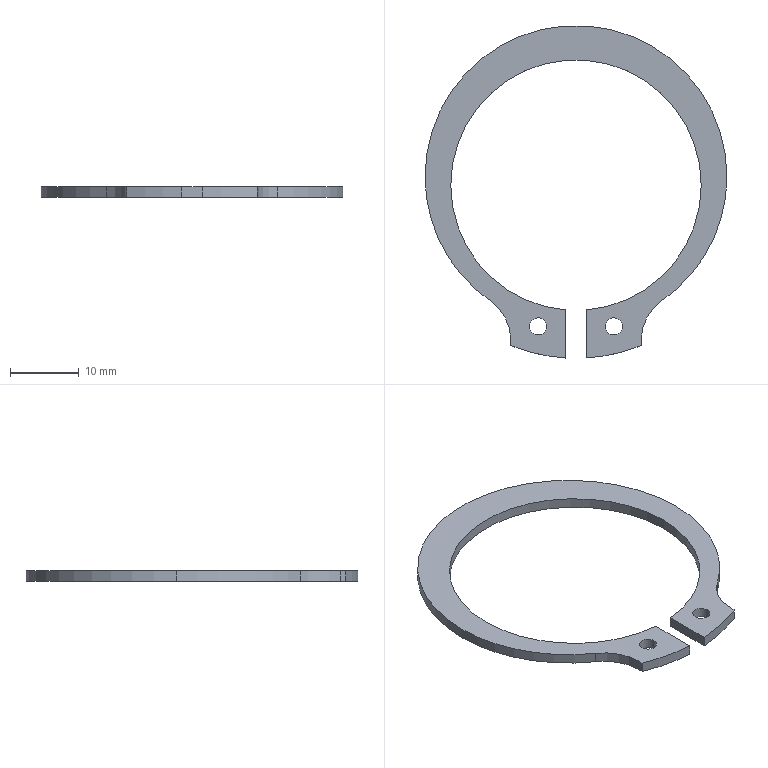Part | SolidWorks | features BaseBody 1 | 1 solid | 20 faces | box 44 x 48.435 x 1.5 mm | volume 802.613 mm3 | cylinder 14 | plane 6 | commonest cylinder face diameters 2.5 x4 36.5 x3 44 x3 14 x2 50.46 x2
STEP:
#1=CARTESIAN_POINT('',(22.,0.,-1.5));
#2=VERTEX_POINT('',#1);
#3=CARTESIAN_POINT('',(-22.,0.,-1.5));
#4=VERTEX_POINT('',#3);
#5=CARTESIAN_POINT('',(0.,0.,-1.5));
#6=DIRECTION('',(0.,0.,1.));
#7=DIRECTION('',(1.,0.,0.));
#8=AXIS2_PLACEMENT_3D('',#5,#6,#7);
#9=CIRCLE('',#8,22.);
#10=EDGE_CURVE('',#2,#4,#9,.T.);
#11=ORIENTED_EDGE('',*,*,#10,.T.);
#12=CARTESIAN_POINT('',(-22.,0.,0.));
#13=VERTEX_POINT('',#12);
#14=CARTESIAN_POINT('',(-22.,0.,-1.5));
#15=DIRECTION('',(0.,0.,1.));
#16=VECTOR('',#15,1000.);
#17=LINE('',#14,#16);
#18=EDGE_CURVE('',#4,#13,#17,.T.);
#19=ORIENTED_EDGE('',*,*,#18,.T.);
#20=CARTESIAN_POINT('',(22.,0.,0.));
#21=VERTEX_POINT('',#20);
#22=CARTESIAN_POINT('',(0.,0.,0.));
#23=DIRECTION('',(0.,0.,-1.));
#24=DIRECTION('',(1.,0.,0.));
#25=AXIS2_PLACEMENT_3D('',#22,#23,#24);
#26=CIRCLE('',#25,22.);
#27=EDGE_CURVE('',#13,#21,#26,.T.);
#28=ORIENTED_EDGE('',*,*,#27,.T.);
#29=CARTESIAN_POINT('',(22.,0.,-1.5));
#30=DIRECTION('',(0.,0.,1.));
#31=VECTOR('',#30,1000.);
#32=LINE('',#29,#31);
#33=EDGE_CURVE('',#2,#21,#32,.T.);
#34=ORIENTED_EDGE('',*,*,#33,.F.);
#35=EDGE_LOOP('',(#11,#19,#28,#34));
#36=FACE_OUTER_BOUND('',#35,.T.);
#37=CARTESIAN_POINT('',(0.,0.,-1.5));
#38=DIRECTION('',(0.,0.,1.));
#39=DIRECTION('',(1.,0.,0.));
#40=AXIS2_PLACEMENT_3D('',#37,#38,#39);
#41=CYLINDRICAL_SURFACE('',#40,22.);
#42=ADVANCED_FACE('',(#36),#41,.T.);
#43=CARTESIAN_POINT('',(12.517,-18.092,-1.5));
#44=VERTEX_POINT('',#43);
#45=CARTESIAN_POINT('',(0.,0.,-1.5));
#46=DIRECTION('',(0.,0.,1.));
#47=DIRECTION('',(1.,0.,0.));
#48=AXIS2_PLACEMENT_3D('',#45,#46,#47);
#49=CIRCLE('',#48,22.);
#50=EDGE_CURVE('',#44,#2,#49,.T.);
#51=ORIENTED_EDGE('',*,*,#50,.T.);
#52=ORIENTED_EDGE('',*,*,#33,.T.);
#53=CARTESIAN_POINT('',(12.517,-18.092,0.));
#54=VERTEX_POINT('',#53);
#55=CARTESIAN_POINT('',(0.,0.,0.));
#56=DIRECTION('',(0.,0.,-1.));
#57=DIRECTION('',(1.,0.,0.));
#58=AXIS2_PLACEMENT_3D('',#55,#56,#57);
#59=CIRCLE('',#58,22.);
#60=EDGE_CURVE('',#21,#54,#59,.T.);
#61=ORIENTED_EDGE('',*,*,#60,.T.);
#62=CARTESIAN_POINT('',(12.517,-18.092,-1.5));
#63=DIRECTION('',(0.,0.,-1.));
#64=VECTOR('',#63,1000.);
#65=LINE('',#62,#64);
#66=EDGE_CURVE('',#54,#44,#65,.T.);
#67=ORIENTED_EDGE('',*,*,#66,.T.);
#68=EDGE_LOOP('',(#51,#52,#61,#67));
#69=FACE_OUTER_BOUND('',#68,.T.);
#70=CARTESIAN_POINT('',(0.,0.,-1.5));
#71=DIRECTION('',(0.,0.,1.));
#72=DIRECTION('',(1.,0.,0.));
#73=AXIS2_PLACEMENT_3D('',#70,#71,#72);
#74=CYLINDRICAL_SURFACE('',#73,22.);
#75=ADVANCED_FACE('',(#69),#74,.T.);
#76=CARTESIAN_POINT('',(-1.5,-19.438,-1.5));
#77=VERTEX_POINT('',#76);
#78=CARTESIAN_POINT('',(-18.25,-1.25,-1.5));
#79=VERTEX_POINT('',#78);
#80=CARTESIAN_POINT('',(0.,-1.25,-1.5));
#81=DIRECTION('',(0.,0.,-1.));
#82=DIRECTION('',(1.,0.,0.));
#83=AXIS2_PLACEMENT_3D('',#80,#81,#82);
#84=CIRCLE('',#83,18.25);
#85=EDGE_CURVE('',#77,#79,#84,.T.);
#86=ORIENTED_EDGE('',*,*,#85,.T.);
#87=CARTESIAN_POINT('',(-18.25,-1.25,0.));
#88=VERTEX_POINT('',#87);
#89=CARTESIAN_POINT('',(-18.25,-1.25,-1.5));
#90=DIRECTION('',(0.,0.,1.));
#91=VECTOR('',#90,1000.);
#92=LINE('',#89,#91);
#93=EDGE_CURVE('',#79,#88,#92,.T.);
#94=ORIENTED_EDGE('',*,*,#93,.T.);
#95=CARTESIAN_POINT('',(-1.5,-19.438,0.));
#96=VERTEX_POINT('',#95);
#97=CARTESIAN_POINT('',(0.,-1.25,0.));
#98=DIRECTION('',(0.,0.,-1.));
#99=DIRECTION('',(1.,0.,0.));
#100=AXIS2_PLACEMENT_3D('',#97,#98,#99);
#101=CIRCLE('',#100,18.25);
#102=EDGE_CURVE('',#96,#88,#101,.T.);
#103=ORIENTED_EDGE('',*,*,#102,.F.);
#104=CARTESIAN_POINT('',(-1.5,-19.438,-1.5));
#105=DIRECTION('',(0.,0.,1.));
#106=VECTOR('',#105,1000.);
#107=LINE('',#104,#106);
#108=EDGE_CURVE('',#77,#96,#107,.T.);
#109=ORIENTED_EDGE('',*,*,#108,.F.);
#110=EDGE_LOOP('',(#86,#94,#103,#109));
#111=FACE_OUTER_BOUND('',#110,.T.);
#112=CARTESIAN_POINT('',(0.,-1.25,-1.5));
#113=DIRECTION('',(0.,0.,1.));
#114=DIRECTION('',(1.,0.,0.));
#115=AXIS2_PLACEMENT_3D('',#112,#113,#114);
#116=CYLINDRICAL_SURFACE('',#115,18.25);
#117=ADVANCED_FACE('',(#111),#116,.F.);
#118=ORIENTED_EDGE('',*,*,#93,.F.);
#119=CARTESIAN_POINT('',(18.25,-1.25,-1.5));
#120=VERTEX_POINT('',#119);
#121=CARTESIAN_POINT('',(0.,-1.25,-1.5));
#122=DIRECTION('',(0.,0.,-1.));
#123=DIRECTION('',(1.,0.,0.));
#124=AXIS2_PLACEMENT_3D('',#121,#122,#123);
#125=CIRCLE('',#124,18.25);
#126=EDGE_CURVE('',#79,#120,#125,.T.);
#127=ORIENTED_EDGE('',*,*,#126,.T.);
#128=CARTESIAN_POINT('',(18.25,-1.25,0.));
#129=VERTEX_POINT('',#128);
#130=CARTESIAN_POINT('',(18.25,-1.25,-1.5));
#131=DIRECTION('',(0.,0.,1.));
#132=VECTOR('',#131,1000.);
#133=LINE('',#130,#132);
#134=EDGE_CURVE('',#120,#129,#133,.T.);
#135=ORIENTED_EDGE('',*,*,#134,.T.);
#136=CARTESIAN_POINT('',(0.,-1.25,0.));
#137=DIRECTION('',(0.,0.,-1.));
#138=DIRECTION('',(1.,0.,0.));
#139=AXIS2_PLACEMENT_3D('',#136,#137,#138);
#140=CIRCLE('',#139,18.25);
#141=EDGE_CURVE('',#88,#129,#140,.T.);
#142=ORIENTED_EDGE('',*,*,#141,.F.);
#143=EDGE_LOOP('',(#118,#127,#135,#142));
#144=FACE_OUTER_BOUND('',#143,.T.);
#145=CARTESIAN_POINT('',(0.,-1.25,-1.5));
#146=DIRECTION('',(0.,0.,1.));
#147=DIRECTION('',(1.,0.,0.));
#148=AXIS2_PLACEMENT_3D('',#145,#146,#147);
#149=CYLINDRICAL_SURFACE('',#148,18.25);
#150=ADVANCED_FACE('',(#144),#149,.F.);
#151=CARTESIAN_POINT('',(-4.25,-21.828,-1.5));
#152=VERTEX_POINT('',#151);
#153=CARTESIAN_POINT('',(-6.75,-21.828,-1.5));
#154=VERTEX_POINT('',#153);
#155=CARTESIAN_POINT('',(-5.5,-21.828,-1.5));
#156=DIRECTION('',(0.,0.,-1.));
#157=DIRECTION('',(1.,0.,0.));
#158=AXIS2_PLACEMENT_3D('',#155,#156,#157);
#159=CIRCLE('',#158,1.25);
#160=EDGE_CURVE('',#152,#154,#159,.T.);
#161=ORIENTED_EDGE('',*,*,#160,.T.);
#162=CARTESIAN_POINT('',(-6.75,-21.828,0.));
#163=VERTEX_POINT('',#162);
#164=CARTESIAN_POINT('',(-6.75,-21.828,-1.5));
#165=DIRECTION('',(0.,0.,1.));
#166=VECTOR('',#165,1000.);
#167=LINE('',#164,#166);
#168=EDGE_CURVE('',#154,#163,#167,.T.);
#169=ORIENTED_EDGE('',*,*,#168,.T.);
#170=CARTESIAN_POINT('',(-4.25,-21.828,0.));
#171=VERTEX_POINT('',#170);
#172=CARTESIAN_POINT('',(-5.5,-21.828,0.));
#173=DIRECTION('',(0.,0.,-1.));
#174=DIRECTION('',(1.,0.,0.));
#175=AXIS2_PLACEMENT_3D('',#172,#173,#174);
#176=CIRCLE('',#175,1.25);
#177=EDGE_CURVE('',#171,#163,#176,.T.);
#178=ORIENTED_EDGE('',*,*,#177,.F.);
#179=CARTESIAN_POINT('',(-4.25,-21.828,-1.5));
#180=DIRECTION('',(0.,0.,1.));
#181=VECTOR('',#180,1000.);
#182=LINE('',#179,#181);
#183=EDGE_CURVE('',#152,#171,#182,.T.);
#184=ORIENTED_EDGE('',*,*,#183,.F.);
#185=EDGE_LOOP('',(#161,#169,#178,#184));
#186=FACE_OUTER_BOUND('',#185,.T.);
#187=CARTESIAN_POINT('',(-5.5,-21.828,-1.5));
#188=DIRECTION('',(0.,0.,1.));
#189=DIRECTION('',(1.,0.,0.));
#190=AXIS2_PLACEMENT_3D('',#187,#188,#189);
#191=CYLINDRICAL_SURFACE('',#190,1.25);
#192=ADVANCED_FACE('',(#186),#191,.F.);
#193=CARTESIAN_POINT('',(6.75,-21.828,-1.5));
#194=VERTEX_POINT('',#193);
#195=CARTESIAN_POINT('',(4.25,-21.828,-1.5));
#196=VERTEX_POINT('',#195);
#197=CARTESIAN_POINT('',(5.5,-21.828,-1.5));
#198=DIRECTION('',(0.,0.,-1.));
#199=DIRECTION('',(1.,0.,0.));
#200=AXIS2_PLACEMENT_3D('',#197,#198,#199);
#201=CIRCLE('',#200,1.25);
#202=EDGE_CURVE('',#194,#196,#201,.T.);
#203=ORIENTED_EDGE('',*,*,#202,.T.);
#204=CARTESIAN_POINT('',(4.25,-21.828,0.));
#205=VERTEX_POINT('',#204);
#206=CARTESIAN_POINT('',(4.25,-21.828,-1.5));
#207=DIRECTION('',(0.,0.,1.));
#208=VECTOR('',#207,1000.);
#209=LINE('',#206,#208);
#210=EDGE_CURVE('',#196,#205,#209,.T.);
#211=ORIENTED_EDGE('',*,*,#210,.T.);
#212=CARTESIAN_POINT('',(6.75,-21.828,0.));
#213=VERTEX_POINT('',#212);
#214=CARTESIAN_POINT('',(5.5,-21.828,0.));
#215=DIRECTION('',(0.,0.,-1.));
#216=DIRECTION('',(1.,0.,0.));
#217=AXIS2_PLACEMENT_3D('',#214,#215,#216);
#218=CIRCLE('',#217,1.25);
#219=EDGE_CURVE('',#213,#205,#218,.T.);
#220=ORIENTED_EDGE('',*,*,#219,.F.);
#221=CARTESIAN_POINT('',(6.75,-21.828,-1.5));
#222=DIRECTION('',(0.,0.,1.));
#223=VECTOR('',#222,1000.);
#224=LINE('',#221,#223);
#225=EDGE_CURVE('',#194,#213,#224,.T.);
#226=ORIENTED_EDGE('',*,*,#225,.F.);
#227=EDGE_LOOP('',(#203,#211,#220,#226));
#228=FACE_OUTER_BOUND('',#227,.T.);
#229=CARTESIAN_POINT('',(5.5,-21.828,-1.5));
#230=DIRECTION('',(0.,0.,1.));
#231=DIRECTION('',(1.,0.,0.));
#232=AXIS2_PLACEMENT_3D('',#229,#230,#231);
#233=CYLINDRICAL_SURFACE('',#232,1.25);
#234=ADVANCED_FACE('',(#228),#233,.F.);
#235=CARTESIAN_POINT('',(9.5,-23.848,-1.5));
#236=VERTEX_POINT('',#235);
#237=CARTESIAN_POINT('',(16.5,-23.848,-1.5));
#238=DIRECTION('',(0.,0.,-1.));
#239=DIRECTION('',(1.,0.,0.));
#240=AXIS2_PLACEMENT_3D('',#237,#238,#239);
#241=CIRCLE('',#240,7.);
#242=EDGE_CURVE('',#236,#44,#241,.T.);
#243=ORIENTED_EDGE('',*,*,#242,.F.);
#244=CARTESIAN_POINT('',(9.5,-24.623,-1.5));
#245=VERTEX_POINT('',#244);
#246=CARTESIAN_POINT('',(9.5,0.,-1.5));
#247=DIRECTION('',(0.,1.,0.));
#248=VECTOR('',#247,1000.);
#249=LINE('',#246,#248);
#250=EDGE_CURVE('',#245,#236,#249,.T.);
#251=ORIENTED_EDGE('',*,*,#250,.F.);
#252=CARTESIAN_POINT('',(1.5,-26.435,-1.5));
#253=VERTEX_POINT('',#252);
#254=CARTESIAN_POINT('',(0.,-1.25,-1.5));
#255=DIRECTION('',(0.,0.,1.));
#256=DIRECTION('',(1.,0.,0.));
#257=AXIS2_PLACEMENT_3D('',#254,#255,#256);
#258=CIRCLE('',#257,25.23);
#259=EDGE_CURVE('',#253,#245,#258,.T.);
#260=ORIENTED_EDGE('',*,*,#259,.F.);
#261=CARTESIAN_POINT('',(1.5,-19.438,-1.5));
#262=VERTEX_POINT('',#261);
#263=CARTESIAN_POINT('',(1.5,0.,-1.5));
#264=DIRECTION('',(0.,-1.,0.));
#265=VECTOR('',#264,1000.);
#266=LINE('',#263,#265);
#267=EDGE_CURVE('',#262,#253,#266,.T.);
#268=ORIENTED_EDGE('',*,*,#267,.F.);
#269=CARTESIAN_POINT('',(0.,-1.25,-1.5));
#270=DIRECTION('',(0.,0.,-1.));
#271=DIRECTION('',(1.,0.,0.));
#272=AXIS2_PLACEMENT_3D('',#269,#270,#271);
#273=CIRCLE('',#272,18.25);
#274=EDGE_CURVE('',#120,#262,#273,.T.);
#275=ORIENTED_EDGE('',*,*,#274,.F.);
#276=ORIENTED_EDGE('',*,*,#126,.F.);
#277=ORIENTED_EDGE('',*,*,#85,.F.);
#278=CARTESIAN_POINT('',(-1.5,-26.435,-1.5));
#279=VERTEX_POINT('',#278);
#280=CARTESIAN_POINT('',(-1.5,0.,-1.5));
#281=DIRECTION('',(0.,1.,0.));
#282=VECTOR('',#281,1000.);
#283=LINE('',#280,#282);
#284=EDGE_CURVE('',#279,#77,#283,.T.);
#285=ORIENTED_EDGE('',*,*,#284,.F.);
#286=CARTESIAN_POINT('',(-9.5,-24.623,-1.5));
#287=VERTEX_POINT('',#286);
#288=CARTESIAN_POINT('',(0.,-1.25,-1.5));
#289=DIRECTION('',(0.,0.,1.));
#290=DIRECTION('',(1.,0.,0.));
#291=AXIS2_PLACEMENT_3D('',#288,#289,#290);
#292=CIRCLE('',#291,25.23);
#293=EDGE_CURVE('',#287,#279,#292,.T.);
#294=ORIENTED_EDGE('',*,*,#293,.F.);
#295=CARTESIAN_POINT('',(-9.5,-23.848,-1.5));
#296=VERTEX_POINT('',#295);
#297=CARTESIAN_POINT('',(-9.5,0.,-1.5));
#298=DIRECTION('',(0.,-1.,0.));
#299=VECTOR('',#298,1000.);
#300=LINE('',#297,#299);
#301=EDGE_CURVE('',#296,#287,#300,.T.);
#302=ORIENTED_EDGE('',*,*,#301,.F.);
#303=CARTESIAN_POINT('',(-12.517,-18.092,-1.5));
#304=VERTEX_POINT('',#303);
#305=CARTESIAN_POINT('',(-16.5,-23.848,-1.5));
#306=DIRECTION('',(0.,0.,-1.));
#307=DIRECTION('',(1.,0.,0.));
#308=AXIS2_PLACEMENT_3D('',#305,#306,#307);
#309=CIRCLE('',#308,7.);
#310=EDGE_CURVE('',#304,#296,#309,.T.);
#311=ORIENTED_EDGE('',*,*,#310,.F.);
#312=CARTESIAN_POINT('',(0.,0.,-1.5));
#313=DIRECTION('',(0.,0.,1.));
#314=DIRECTION('',(1.,0.,0.));
#315=AXIS2_PLACEMENT_3D('',#312,#313,#314);
#316=CIRCLE('',#315,22.);
#317=EDGE_CURVE('',#4,#304,#316,.T.);
#318=ORIENTED_EDGE('',*,*,#317,.F.);
#319=ORIENTED_EDGE('',*,*,#10,.F.);
#320=ORIENTED_EDGE('',*,*,#50,.F.);
#321=EDGE_LOOP('',(#243,#251,#260,#268,#275,#276,#277,#285,#294,#302,#311,#318,#319,#320));
#322=FACE_OUTER_BOUND('',#321,.T.);
#323=ORIENTED_EDGE('',*,*,#160,.F.);
#324=CARTESIAN_POINT('',(-5.5,-21.828,-1.5));
#325=DIRECTION('',(0.,0.,-1.));
#326=DIRECTION('',(1.,0.,0.));
#327=AXIS2_PLACEMENT_3D('',#324,#325,#326);
#328=CIRCLE('',#327,1.25);
#329=EDGE_CURVE('',#154,#152,#328,.T.);
#330=ORIENTED_EDGE('',*,*,#329,.F.);
#331=EDGE_LOOP('',(#323,#330));
#332=FACE_BOUND('',#331,.T.);
#333=ORIENTED_EDGE('',*,*,#202,.F.);
#334=CARTESIAN_POINT('',(5.5,-21.828,-1.5));
#335=DIRECTION('',(0.,0.,-1.));
#336=DIRECTION('',(1.,0.,0.));
#337=AXIS2_PLACEMENT_3D('',#334,#335,#336);
#338=CIRCLE('',#337,1.25);
#339=EDGE_CURVE('',#196,#194,#338,.T.);
#340=ORIENTED_EDGE('',*,*,#339,.F.);
#341=EDGE_LOOP('',(#333,#340));
#342=FACE_BOUND('',#341,.T.);
#343=CARTESIAN_POINT('',(0.,0.,-1.5));
#344=DIRECTION('',(0.,0.,1.));
#345=DIRECTION('',(1.,0.,0.));
#346=AXIS2_PLACEMENT_3D('',#343,#344,#345);
#347=PLANE('',#346);
#348=ADVANCED_FACE('',(#322,#332,#342),#347,.F.);
#349=ORIENTED_EDGE('',*,*,#18,.F.);
#350=ORIENTED_EDGE('',*,*,#317,.T.);
#351=CARTESIAN_POINT('',(-12.517,-18.092,0.));
#352=VERTEX_POINT('',#351);
#353=CARTESIAN_POINT('',(-12.517,-18.092,-1.5));
#354=DIRECTION('',(0.,0.,1.));
#355=VECTOR('',#354,1000.);
#356=LINE('',#353,#355);
#357=EDGE_CURVE('',#304,#352,#356,.T.);
#358=ORIENTED_EDGE('',*,*,#357,.T.);
#359=CARTESIAN_POINT('',(0.,0.,0.));
#360=DIRECTION('',(0.,0.,-1.));
#361=DIRECTION('',(1.,0.,0.));
#362=AXIS2_PLACEMENT_3D('',#359,#360,#361);
#363=CIRCLE('',#362,22.);
#364=EDGE_CURVE('',#352,#13,#363,.T.);
#365=ORIENTED_EDGE('',*,*,#364,.T.);
#366=EDGE_LOOP('',(#349,#350,#358,#365));
#367=FACE_OUTER_BOUND('',#366,.T.);
#368=CARTESIAN_POINT('',(0.,0.,-1.5));
#369=DIRECTION('',(0.,0.,1.));
#370=DIRECTION('',(1.,0.,0.));
#371=AXIS2_PLACEMENT_3D('',#368,#369,#370);
#372=CYLINDRICAL_SURFACE('',#371,22.);
#373=ADVANCED_FACE('',(#367),#372,.T.);
#374=ORIENTED_EDGE('',*,*,#66,.F.);
#375=CARTESIAN_POINT('',(9.5,-23.848,0.));
#376=VERTEX_POINT('',#375);
#377=CARTESIAN_POINT('',(16.5,-23.848,0.));
#378=DIRECTION('',(0.,0.,-1.));
#379=DIRECTION('',(1.,0.,0.));
#380=AXIS2_PLACEMENT_3D('',#377,#378,#379);
#381=CIRCLE('',#380,7.);
#382=EDGE_CURVE('',#376,#54,#381,.T.);
#383=ORIENTED_EDGE('',*,*,#382,.F.);
#384=CARTESIAN_POINT('',(9.5,-23.848,-1.5));
#385=DIRECTION('',(0.,0.,1.));
#386=VECTOR('',#385,1000.);
#387=LINE('',#384,#386);
#388=EDGE_CURVE('',#236,#376,#387,.T.);
#389=ORIENTED_EDGE('',*,*,#388,.F.);
#390=ORIENTED_EDGE('',*,*,#242,.T.);
#391=EDGE_LOOP('',(#374,#383,#389,#390));
#392=FACE_OUTER_BOUND('',#391,.T.);
#393=CARTESIAN_POINT('',(16.5,-23.848,-1.5));
#394=DIRECTION('',(0.,0.,1.));
#395=DIRECTION('',(1.,0.,0.));
#396=AXIS2_PLACEMENT_3D('',#393,#394,#395);
#397=CYLINDRICAL_SURFACE('',#396,7.);
#398=ADVANCED_FACE('',(#392),#397,.F.);
#399=CARTESIAN_POINT('',(9.5,-24.623,0.));
#400=VERTEX_POINT('',#399);
#401=CARTESIAN_POINT('',(9.5,-19.843,0.));
#402=DIRECTION('',(0.,-1.,0.));
#403=VECTOR('',#402,1000.);
#404=LINE('',#401,#403);
#405=EDGE_CURVE('',#376,#400,#404,.T.);
#406=ORIENTED_EDGE('',*,*,#405,.T.);
#407=CARTESIAN_POINT('',(9.5,-24.623,-1.5));
#408=DIRECTION('',(0.,0.,-1.));
#409=VECTOR('',#408,1000.);
#410=LINE('',#407,#409);
#411=EDGE_CURVE('',#400,#245,#410,.T.);
#412=ORIENTED_EDGE('',*,*,#411,.T.);
#413=ORIENTED_EDGE('',*,*,#250,.T.);
#414=ORIENTED_EDGE('',*,*,#388,.T.);
#415=EDGE_LOOP('',(#406,#412,#413,#414));
#416=FACE_OUTER_BOUND('',#415,.T.);
#417=CARTESIAN_POINT('',(9.5,-19.843,-1.5));
#418=DIRECTION('',(1.,0.,0.));
#419=DIRECTION('',(0.,1.,0.));
#420=AXIS2_PLACEMENT_3D('',#417,#418,#419);
#421=PLANE('',#420);
#422=ADVANCED_FACE('',(#416),#421,.T.);
#423=ORIENTED_EDGE('',*,*,#259,.T.);
#424=ORIENTED_EDGE('',*,*,#411,.F.);
#425=CARTESIAN_POINT('',(1.5,-26.435,0.));
#426=VERTEX_POINT('',#425);
#427=CARTESIAN_POINT('',(0.,-1.25,0.));
#428=DIRECTION('',(0.,0.,-1.));
#429=DIRECTION('',(1.,0.,0.));
#430=AXIS2_PLACEMENT_3D('',#427,#428,#429);
#431=CIRCLE('',#430,25.23);
#432=EDGE_CURVE('',#400,#426,#431,.T.);
#433=ORIENTED_EDGE('',*,*,#432,.T.);
#434=CARTESIAN_POINT('',(1.5,-26.435,-1.5));
#435=DIRECTION('',(0.,0.,-1.));
#436=VECTOR('',#435,1000.);
#437=LINE('',#434,#436);
#438=EDGE_CURVE('',#426,#253,#437,.T.);
#439=ORIENTED_EDGE('',*,*,#438,.T.);
#440=EDGE_LOOP('',(#423,#424,#433,#439));
#441=FACE_OUTER_BOUND('',#440,.T.);
#442=CARTESIAN_POINT('',(0.,-1.25,-1.5));
#443=DIRECTION('',(0.,0.,1.));
#444=DIRECTION('',(1.,0.,0.));
#445=AXIS2_PLACEMENT_3D('',#442,#443,#444);
#446=CYLINDRICAL_SURFACE('',#445,25.23);
#447=ADVANCED_FACE('',(#441),#446,.T.);
#448=ORIENTED_EDGE('',*,*,#267,.T.);
#449=ORIENTED_EDGE('',*,*,#438,.F.);
#450=CARTESIAN_POINT('',(1.5,-19.438,0.));
#451=VERTEX_POINT('',#450);
#452=CARTESIAN_POINT('',(1.5,-26.435,0.));
#453=DIRECTION('',(0.,1.,0.));
#454=VECTOR('',#453,1000.);
#455=LINE('',#452,#454);
#456=EDGE_CURVE('',#426,#451,#455,.T.);
#457=ORIENTED_EDGE('',*,*,#456,.T.);
#458=CARTESIAN_POINT('',(1.5,-19.438,-1.5));
#459=DIRECTION('',(0.,0.,-1.));
#460=VECTOR('',#459,1000.);
#461=LINE('',#458,#460);
#462=EDGE_CURVE('',#451,#262,#461,.T.);
#463=ORIENTED_EDGE('',*,*,#462,.T.);
#464=EDGE_LOOP('',(#448,#449,#457,#463));
#465=FACE_OUTER_BOUND('',#464,.T.);
#466=CARTESIAN_POINT('',(1.5,-26.435,-1.5));
#467=DIRECTION('',(-1.,0.,0.));
#468=DIRECTION('',(0.,-1.,0.));
#469=AXIS2_PLACEMENT_3D('',#466,#467,#468);
#470=PLANE('',#469);
#471=ADVANCED_FACE('',(#465),#470,.T.);
#472=ORIENTED_EDGE('',*,*,#134,.F.);
#473=ORIENTED_EDGE('',*,*,#274,.T.);
#474=ORIENTED_EDGE('',*,*,#462,.F.);
#475=CARTESIAN_POINT('',(0.,-1.25,0.));
#476=DIRECTION('',(0.,0.,-1.));
#477=DIRECTION('',(1.,0.,0.));
#478=AXIS2_PLACEMENT_3D('',#475,#476,#477);
#479=CIRCLE('',#478,18.25);
#480=EDGE_CURVE('',#129,#451,#479,.T.);
#481=ORIENTED_EDGE('',*,*,#480,.F.);
#482=EDGE_LOOP('',(#472,#473,#474,#481));
#483=FACE_OUTER_BOUND('',#482,.T.);
#484=CARTESIAN_POINT('',(0.,-1.25,-1.5));
#485=DIRECTION('',(0.,0.,1.));
#486=DIRECTION('',(1.,0.,0.));
#487=AXIS2_PLACEMENT_3D('',#484,#485,#486);
#488=CYLINDRICAL_SURFACE('',#487,18.25);
#489=ADVANCED_FACE('',(#483),#488,.F.);
#490=ORIENTED_EDGE('',*,*,#284,.T.);
#491=ORIENTED_EDGE('',*,*,#108,.T.);
#492=CARTESIAN_POINT('',(-1.5,-26.435,0.));
#493=VERTEX_POINT('',#492);
#494=CARTESIAN_POINT('',(-1.5,-26.435,0.));
#495=DIRECTION('',(0.,-1.,0.));
#496=VECTOR('',#495,1000.);
#497=LINE('',#494,#496);
#498=EDGE_CURVE('',#96,#493,#497,.T.);
#499=ORIENTED_EDGE('',*,*,#498,.T.);
#500=CARTESIAN_POINT('',(-1.5,-26.435,-1.5));
#501=DIRECTION('',(0.,0.,-1.));
#502=VECTOR('',#501,1000.);
#503=LINE('',#500,#502);
#504=EDGE_CURVE('',#493,#279,#503,.T.);
#505=ORIENTED_EDGE('',*,*,#504,.T.);
#506=EDGE_LOOP('',(#490,#491,#499,#505));
#507=FACE_OUTER_BOUND('',#506,.T.);
#508=CARTESIAN_POINT('',(-1.5,-26.435,-1.5));
#509=DIRECTION('',(1.,0.,0.));
#510=DIRECTION('',(0.,1.,0.));
#511=AXIS2_PLACEMENT_3D('',#508,#509,#510);
#512=PLANE('',#511);
#513=ADVANCED_FACE('',(#507),#512,.T.);
#514=ORIENTED_EDGE('',*,*,#293,.T.);
#515=ORIENTED_EDGE('',*,*,#504,.F.);
#516=CARTESIAN_POINT('',(-9.5,-24.623,0.));
#517=VERTEX_POINT('',#516);
#518=CARTESIAN_POINT('',(0.,-1.25,0.));
#519=DIRECTION('',(0.,0.,-1.));
#520=DIRECTION('',(1.,0.,0.));
#521=AXIS2_PLACEMENT_3D('',#518,#519,#520);
#522=CIRCLE('',#521,25.23);
#523=EDGE_CURVE('',#493,#517,#522,.T.);
#524=ORIENTED_EDGE('',*,*,#523,.T.);
#525=CARTESIAN_POINT('',(-9.5,-24.623,-1.5));
#526=DIRECTION('',(0.,0.,-1.));
#527=VECTOR('',#526,1000.);
#528=LINE('',#525,#527);
#529=EDGE_CURVE('',#517,#287,#528,.T.);
#530=ORIENTED_EDGE('',*,*,#529,.T.);
#531=EDGE_LOOP('',(#514,#515,#524,#530));
#532=FACE_OUTER_BOUND('',#531,.T.);
#533=CARTESIAN_POINT('',(0.,-1.25,-1.5));
#534=DIRECTION('',(0.,0.,1.));
#535=DIRECTION('',(1.,0.,0.));
#536=AXIS2_PLACEMENT_3D('',#533,#534,#535);
#537=CYLINDRICAL_SURFACE('',#536,25.23);
#538=ADVANCED_FACE('',(#532),#537,.T.);
#539=ORIENTED_EDGE('',*,*,#301,.T.);
#540=ORIENTED_EDGE('',*,*,#529,.F.);
#541=CARTESIAN_POINT('',(-9.5,-23.848,0.));
#542=VERTEX_POINT('',#541);
#543=CARTESIAN_POINT('',(-9.5,-19.843,0.));
#544=DIRECTION('',(0.,1.,0.));
#545=VECTOR('',#544,1000.);
#546=LINE('',#543,#545);
#547=EDGE_CURVE('',#517,#542,#546,.T.);
#548=ORIENTED_EDGE('',*,*,#547,.T.);
#549=CARTESIAN_POINT('',(-9.5,-23.848,-1.5));
#550=DIRECTION('',(0.,0.,-1.));
#551=VECTOR('',#550,1000.);
#552=LINE('',#549,#551);
#553=EDGE_CURVE('',#542,#296,#552,.T.);
#554=ORIENTED_EDGE('',*,*,#553,.T.);
#555=EDGE_LOOP('',(#539,#540,#548,#554));
#556=FACE_OUTER_BOUND('',#555,.T.);
#557=CARTESIAN_POINT('',(-9.5,-19.843,-1.5));
#558=DIRECTION('',(-1.,0.,0.));
#559=DIRECTION('',(0.,-1.,0.));
#560=AXIS2_PLACEMENT_3D('',#557,#558,#559);
#561=PLANE('',#560);
#562=ADVANCED_FACE('',(#556),#561,.T.);
#563=ORIENTED_EDGE('',*,*,#553,.F.);
#564=CARTESIAN_POINT('',(-16.5,-23.848,0.));
#565=DIRECTION('',(0.,0.,-1.));
#566=DIRECTION('',(1.,0.,0.));
#567=AXIS2_PLACEMENT_3D('',#564,#565,#566);
#568=CIRCLE('',#567,7.);
#569=EDGE_CURVE('',#352,#542,#568,.T.);
#570=ORIENTED_EDGE('',*,*,#569,.F.);
#571=ORIENTED_EDGE('',*,*,#357,.F.);
#572=ORIENTED_EDGE('',*,*,#310,.T.);
#573=EDGE_LOOP('',(#563,#570,#571,#572));
#574=FACE_OUTER_BOUND('',#573,.T.);
#575=CARTESIAN_POINT('',(-16.5,-23.848,-1.5));
#576=DIRECTION('',(0.,0.,1.));
#577=DIRECTION('',(1.,0.,0.));
#578=AXIS2_PLACEMENT_3D('',#575,#576,#577);
#579=CYLINDRICAL_SURFACE('',#578,7.);
#580=ADVANCED_FACE('',(#574),#579,.F.);
#581=ORIENTED_EDGE('',*,*,#168,.F.);
#582=ORIENTED_EDGE('',*,*,#329,.T.);
#583=ORIENTED_EDGE('',*,*,#183,.T.);
#584=CARTESIAN_POINT('',(-5.5,-21.828,0.));
#585=DIRECTION('',(0.,0.,-1.));
#586=DIRECTION('',(1.,0.,0.));
#587=AXIS2_PLACEMENT_3D('',#584,#585,#586);
#588=CIRCLE('',#587,1.25);
#589=EDGE_CURVE('',#163,#171,#588,.T.);
#590=ORIENTED_EDGE('',*,*,#589,.F.);
#591=EDGE_LOOP('',(#581,#582,#583,#590));
#592=FACE_OUTER_BOUND('',#591,.T.);
#593=CARTESIAN_POINT('',(-5.5,-21.828,-1.5));
#594=DIRECTION('',(0.,0.,1.));
#595=DIRECTION('',(1.,0.,0.));
#596=AXIS2_PLACEMENT_3D('',#593,#594,#595);
#597=CYLINDRICAL_SURFACE('',#596,1.25);
#598=ADVANCED_FACE('',(#592),#597,.F.);
#599=ORIENTED_EDGE('',*,*,#210,.F.);
#600=ORIENTED_EDGE('',*,*,#339,.T.);
#601=ORIENTED_EDGE('',*,*,#225,.T.);
#602=CARTESIAN_POINT('',(5.5,-21.828,0.));
#603=DIRECTION('',(0.,0.,-1.));
#604=DIRECTION('',(1.,0.,0.));
#605=AXIS2_PLACEMENT_3D('',#602,#603,#604);
#606=CIRCLE('',#605,1.25);
#607=EDGE_CURVE('',#205,#213,#606,.T.);
#608=ORIENTED_EDGE('',*,*,#607,.F.);
#609=EDGE_LOOP('',(#599,#600,#601,#608));
#610=FACE_OUTER_BOUND('',#609,.T.);
#611=CARTESIAN_POINT('',(5.5,-21.828,-1.5));
#612=DIRECTION('',(0.,0.,1.));
#613=DIRECTION('',(1.,0.,0.));
#614=AXIS2_PLACEMENT_3D('',#611,#612,#613);
#615=CYLINDRICAL_SURFACE('',#614,1.25);
#616=ADVANCED_FACE('',(#610),#615,.F.);
#617=ORIENTED_EDGE('',*,*,#456,.F.);
#618=ORIENTED_EDGE('',*,*,#432,.F.);
#619=ORIENTED_EDGE('',*,*,#405,.F.);
#620=ORIENTED_EDGE('',*,*,#382,.T.);
#621=ORIENTED_EDGE('',*,*,#60,.F.);
#622=ORIENTED_EDGE('',*,*,#27,.F.);
#623=ORIENTED_EDGE('',*,*,#364,.F.);
#624=ORIENTED_EDGE('',*,*,#569,.T.);
#625=ORIENTED_EDGE('',*,*,#547,.F.);
#626=ORIENTED_EDGE('',*,*,#523,.F.);
#627=ORIENTED_EDGE('',*,*,#498,.F.);
#628=ORIENTED_EDGE('',*,*,#102,.T.);
#629=ORIENTED_EDGE('',*,*,#141,.T.);
#630=ORIENTED_EDGE('',*,*,#480,.T.);
#631=EDGE_LOOP('',(#617,#618,#619,#620,#621,#622,#623,#624,#625,#626,#627,#628,#629,#630));
#632=FACE_OUTER_BOUND('',#631,.T.);
#633=ORIENTED_EDGE('',*,*,#177,.T.);
#634=ORIENTED_EDGE('',*,*,#589,.T.);
#635=EDGE_LOOP('',(#633,#634));
#636=FACE_BOUND('',#635,.T.);
#637=ORIENTED_EDGE('',*,*,#219,.T.);
#638=ORIENTED_EDGE('',*,*,#607,.T.);
#639=EDGE_LOOP('',(#637,#638));
#640=FACE_BOUND('',#639,.T.);
#641=CARTESIAN_POINT('',(0.,0.,0.));
#642=DIRECTION('',(0.,0.,1.));
#643=DIRECTION('',(1.,0.,0.));
#644=AXIS2_PLACEMENT_3D('',#641,#642,#643);
#645=PLANE('',#644);
#646=ADVANCED_FACE('',(#632,#636,#640),#645,.T.);
#647=CLOSED_SHELL('',(#42,#75,#117,#150,#192,#234,#348,#373,#398,#422,#447,#471,#489,#513,#538,#562,#580,#598,#616,#646));
#648=MANIFOLD_SOLID_BREP('',#647);
#649=CARTESIAN_POINT('',(0.,0.,0.));
#650=DIRECTION('',(0.,0.,1.));
#651=DIRECTION('',(1.,0.,0.));
#652=AXIS2_PLACEMENT_3D('',#649,#650,#651);
#653=(LENGTH_UNIT()NAMED_UNIT(*)SI_UNIT(.MILLI.,.METRE.));
#654=UNCERTAINTY_MEASURE_WITH_UNIT(LENGTH_MEASURE(0.00001),#653,'','');
#655=(NAMED_UNIT(*)PLANE_ANGLE_UNIT()SI_UNIT($,.RADIAN.));
#656=(NAMED_UNIT(*)SI_UNIT($,.STERADIAN.)SOLID_ANGLE_UNIT());
#657=(GEOMETRIC_REPRESENTATION_CONTEXT(3)GLOBAL_UNCERTAINTY_ASSIGNED_CONTEXT((#654))GLOBAL_UNIT_ASSIGNED_CONTEXT((#653,#655,#656))REPRESENTATION_CONTEXT('',''));
#658=ADVANCED_BREP_SHAPE_REPRESENTATION('',(#648,#652),#657);